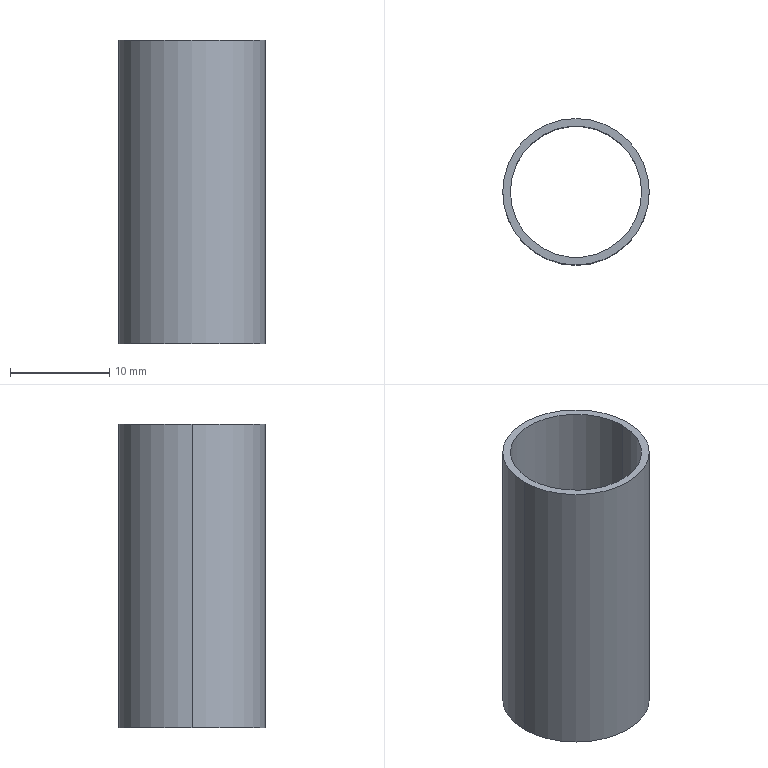Part | SolidWorks | features Extrusion 1, Scale 1 | 1 solid | 6 faces | box 14.732 x 14.732 x 30.48 mm | volume 1019 mm3 | cylinder 4 | plane 2 | commonest cylinder face diameters 13.208 x2 14.732 x2
STEP:
#1=CARTESIAN_POINT('',(-6.604,0.,30.48));
#2=VERTEX_POINT('',#1);
#3=CARTESIAN_POINT('',(6.604,0.,30.48));
#4=VERTEX_POINT('',#3);
#5=CARTESIAN_POINT('',(0.,0.,30.48));
#6=DIRECTION('',(0.,0.,1.));
#7=DIRECTION('',(1.,0.,0.));
#8=AXIS2_PLACEMENT_3D('',#5,#6,#7);
#9=CIRCLE('',#8,6.604);
#10=EDGE_CURVE('',#2,#4,#9,.T.);
#11=ORIENTED_EDGE('',*,*,#10,.T.);
#12=CARTESIAN_POINT('',(6.604,0.,0.));
#13=VERTEX_POINT('',#12);
#14=CARTESIAN_POINT('',(6.604,0.,30.48));
#15=DIRECTION('',(0.,0.,-1.));
#16=VECTOR('',#15,1000.);
#17=LINE('',#14,#16);
#18=EDGE_CURVE('',#4,#13,#17,.T.);
#19=ORIENTED_EDGE('',*,*,#18,.T.);
#20=CARTESIAN_POINT('',(-6.604,0.,0.));
#21=VERTEX_POINT('',#20);
#22=CARTESIAN_POINT('',(0.,0.,0.));
#23=DIRECTION('',(0.,0.,1.));
#24=DIRECTION('',(1.,0.,0.));
#25=AXIS2_PLACEMENT_3D('',#22,#23,#24);
#26=CIRCLE('',#25,6.604);
#27=EDGE_CURVE('',#21,#13,#26,.T.);
#28=ORIENTED_EDGE('',*,*,#27,.F.);
#29=CARTESIAN_POINT('',(-6.604,0.,30.48));
#30=DIRECTION('',(0.,0.,-1.));
#31=VECTOR('',#30,1000.);
#32=LINE('',#29,#31);
#33=EDGE_CURVE('',#2,#21,#32,.T.);
#34=ORIENTED_EDGE('',*,*,#33,.F.);
#35=EDGE_LOOP('',(#11,#19,#28,#34));
#36=FACE_OUTER_BOUND('',#35,.T.);
#37=CARTESIAN_POINT('',(0.,0.,30.48));
#38=DIRECTION('',(0.,0.,-1.));
#39=DIRECTION('',(-1.,0.,0.));
#40=AXIS2_PLACEMENT_3D('',#37,#38,#39);
#41=CYLINDRICAL_SURFACE('',#40,6.604);
#42=ADVANCED_FACE('',(#36),#41,.F.);
#43=CARTESIAN_POINT('',(7.366,0.,30.48));
#44=VERTEX_POINT('',#43);
#45=CARTESIAN_POINT('',(-7.366,0.,30.48));
#46=VERTEX_POINT('',#45);
#47=CARTESIAN_POINT('',(0.,0.,30.48));
#48=DIRECTION('',(0.,0.,1.));
#49=DIRECTION('',(1.,0.,0.));
#50=AXIS2_PLACEMENT_3D('',#47,#48,#49);
#51=CIRCLE('',#50,7.366);
#52=EDGE_CURVE('',#44,#46,#51,.T.);
#53=ORIENTED_EDGE('',*,*,#52,.F.);
#54=CARTESIAN_POINT('',(7.366,0.,0.));
#55=VERTEX_POINT('',#54);
#56=CARTESIAN_POINT('',(7.366,0.,30.48));
#57=DIRECTION('',(0.,0.,-1.));
#58=VECTOR('',#57,1000.);
#59=LINE('',#56,#58);
#60=EDGE_CURVE('',#44,#55,#59,.T.);
#61=ORIENTED_EDGE('',*,*,#60,.T.);
#62=CARTESIAN_POINT('',(-7.366,0.,0.));
#63=VERTEX_POINT('',#62);
#64=CARTESIAN_POINT('',(0.,0.,0.));
#65=DIRECTION('',(0.,0.,1.));
#66=DIRECTION('',(1.,0.,0.));
#67=AXIS2_PLACEMENT_3D('',#64,#65,#66);
#68=CIRCLE('',#67,7.366);
#69=EDGE_CURVE('',#55,#63,#68,.T.);
#70=ORIENTED_EDGE('',*,*,#69,.T.);
#71=CARTESIAN_POINT('',(-7.366,0.,30.48));
#72=DIRECTION('',(0.,0.,-1.));
#73=VECTOR('',#72,1000.);
#74=LINE('',#71,#73);
#75=EDGE_CURVE('',#46,#63,#74,.T.);
#76=ORIENTED_EDGE('',*,*,#75,.F.);
#77=EDGE_LOOP('',(#53,#61,#70,#76));
#78=FACE_OUTER_BOUND('',#77,.T.);
#79=CARTESIAN_POINT('',(0.,0.,30.48));
#80=DIRECTION('',(0.,0.,-1.));
#81=DIRECTION('',(-1.,0.,0.));
#82=AXIS2_PLACEMENT_3D('',#79,#80,#81);
#83=CYLINDRICAL_SURFACE('',#82,7.366);
#84=ADVANCED_FACE('',(#78),#83,.T.);
#85=CARTESIAN_POINT('',(0.,0.,30.48));
#86=DIRECTION('',(0.,0.,1.));
#87=DIRECTION('',(1.,0.,0.));
#88=AXIS2_PLACEMENT_3D('',#85,#86,#87);
#89=CIRCLE('',#88,7.366);
#90=EDGE_CURVE('',#46,#44,#89,.T.);
#91=ORIENTED_EDGE('',*,*,#90,.T.);
#92=ORIENTED_EDGE('',*,*,#52,.T.);
#93=EDGE_LOOP('',(#91,#92));
#94=FACE_OUTER_BOUND('',#93,.T.);
#95=ORIENTED_EDGE('',*,*,#10,.F.);
#96=CARTESIAN_POINT('',(0.,0.,30.48));
#97=DIRECTION('',(0.,0.,1.));
#98=DIRECTION('',(1.,0.,0.));
#99=AXIS2_PLACEMENT_3D('',#96,#97,#98);
#100=CIRCLE('',#99,6.604);
#101=EDGE_CURVE('',#4,#2,#100,.T.);
#102=ORIENTED_EDGE('',*,*,#101,.F.);
#103=EDGE_LOOP('',(#95,#102));
#104=FACE_BOUND('',#103,.T.);
#105=CARTESIAN_POINT('',(0.,0.,30.48));
#106=DIRECTION('',(0.,0.,1.));
#107=DIRECTION('',(1.,0.,0.));
#108=AXIS2_PLACEMENT_3D('',#105,#106,#107);
#109=PLANE('',#108);
#110=ADVANCED_FACE('',(#94,#104),#109,.T.);
#111=CARTESIAN_POINT('',(0.,0.,0.));
#112=DIRECTION('',(0.,0.,1.));
#113=DIRECTION('',(1.,0.,0.));
#114=AXIS2_PLACEMENT_3D('',#111,#112,#113);
#115=CIRCLE('',#114,7.366);
#116=EDGE_CURVE('',#63,#55,#115,.T.);
#117=ORIENTED_EDGE('',*,*,#116,.F.);
#118=ORIENTED_EDGE('',*,*,#69,.F.);
#119=EDGE_LOOP('',(#117,#118));
#120=FACE_OUTER_BOUND('',#119,.T.);
#121=ORIENTED_EDGE('',*,*,#27,.T.);
#122=CARTESIAN_POINT('',(0.,0.,0.));
#123=DIRECTION('',(0.,0.,1.));
#124=DIRECTION('',(1.,0.,0.));
#125=AXIS2_PLACEMENT_3D('',#122,#123,#124);
#126=CIRCLE('',#125,6.604);
#127=EDGE_CURVE('',#13,#21,#126,.T.);
#128=ORIENTED_EDGE('',*,*,#127,.T.);
#129=EDGE_LOOP('',(#121,#128));
#130=FACE_BOUND('',#129,.T.);
#131=CARTESIAN_POINT('',(0.,0.,0.));
#132=DIRECTION('',(0.,0.,1.));
#133=DIRECTION('',(1.,0.,0.));
#134=AXIS2_PLACEMENT_3D('',#131,#132,#133);
#135=PLANE('',#134);
#136=ADVANCED_FACE('',(#120,#130),#135,.F.);
#137=ORIENTED_EDGE('',*,*,#60,.F.);
#138=ORIENTED_EDGE('',*,*,#90,.F.);
#139=ORIENTED_EDGE('',*,*,#75,.T.);
#140=ORIENTED_EDGE('',*,*,#116,.T.);
#141=EDGE_LOOP('',(#137,#138,#139,#140));
#142=FACE_OUTER_BOUND('',#141,.T.);
#143=CARTESIAN_POINT('',(0.,0.,30.48));
#144=DIRECTION('',(0.,0.,-1.));
#145=DIRECTION('',(-1.,0.,0.));
#146=AXIS2_PLACEMENT_3D('',#143,#144,#145);
#147=CYLINDRICAL_SURFACE('',#146,7.366);
#148=ADVANCED_FACE('',(#142),#147,.T.);
#149=ORIENTED_EDGE('',*,*,#18,.F.);
#150=ORIENTED_EDGE('',*,*,#101,.T.);
#151=ORIENTED_EDGE('',*,*,#33,.T.);
#152=ORIENTED_EDGE('',*,*,#127,.F.);
#153=EDGE_LOOP('',(#149,#150,#151,#152));
#154=FACE_OUTER_BOUND('',#153,.T.);
#155=CARTESIAN_POINT('',(0.,0.,30.48));
#156=DIRECTION('',(0.,0.,-1.));
#157=DIRECTION('',(-1.,0.,0.));
#158=AXIS2_PLACEMENT_3D('',#155,#156,#157);
#159=CYLINDRICAL_SURFACE('',#158,6.604);
#160=ADVANCED_FACE('',(#154),#159,.F.);
#161=CLOSED_SHELL('',(#42,#84,#110,#136,#148,#160));
#162=MANIFOLD_SOLID_BREP('',#161);
#163=CARTESIAN_POINT('',(0.,0.,0.));
#164=DIRECTION('',(0.,0.,1.));
#165=DIRECTION('',(1.,0.,0.));
#166=AXIS2_PLACEMENT_3D('',#163,#164,#165);
#167=(LENGTH_UNIT()NAMED_UNIT(*)SI_UNIT(.MILLI.,.METRE.));
#168=UNCERTAINTY_MEASURE_WITH_UNIT(LENGTH_MEASURE(0.00001),#167,'','');
#169=(NAMED_UNIT(*)PLANE_ANGLE_UNIT()SI_UNIT($,.RADIAN.));
#170=(NAMED_UNIT(*)SI_UNIT($,.STERADIAN.)SOLID_ANGLE_UNIT());
#171=(GEOMETRIC_REPRESENTATION_CONTEXT(3)GLOBAL_UNCERTAINTY_ASSIGNED_CONTEXT((#168))GLOBAL_UNIT_ASSIGNED_CONTEXT((#167,#169,#170))REPRESENTATION_CONTEXT('',''));
#172=ADVANCED_BREP_SHAPE_REPRESENTATION('',(#162,#166),#171);